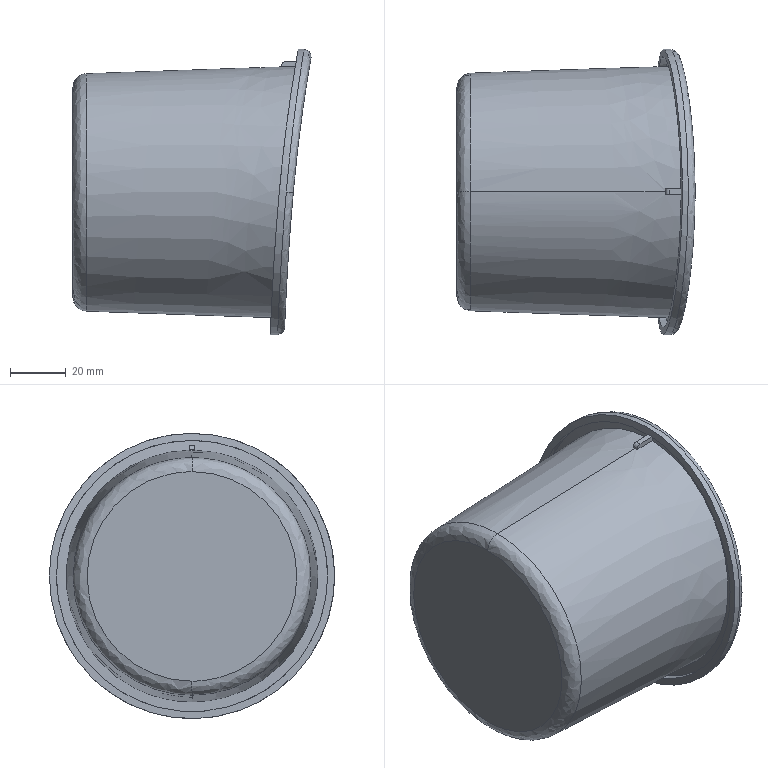Part | STEP file | MANIFOLD_SOLID_BREP_178783_1_1 | 1 solid | 28 faces | box 85.183 x 102 x 102 mm | volume 73233 mm3 | spline 19 | plane 6 | cylinder 3 | commonest cylinder face diameters 3 x1 97 x1 102 x1